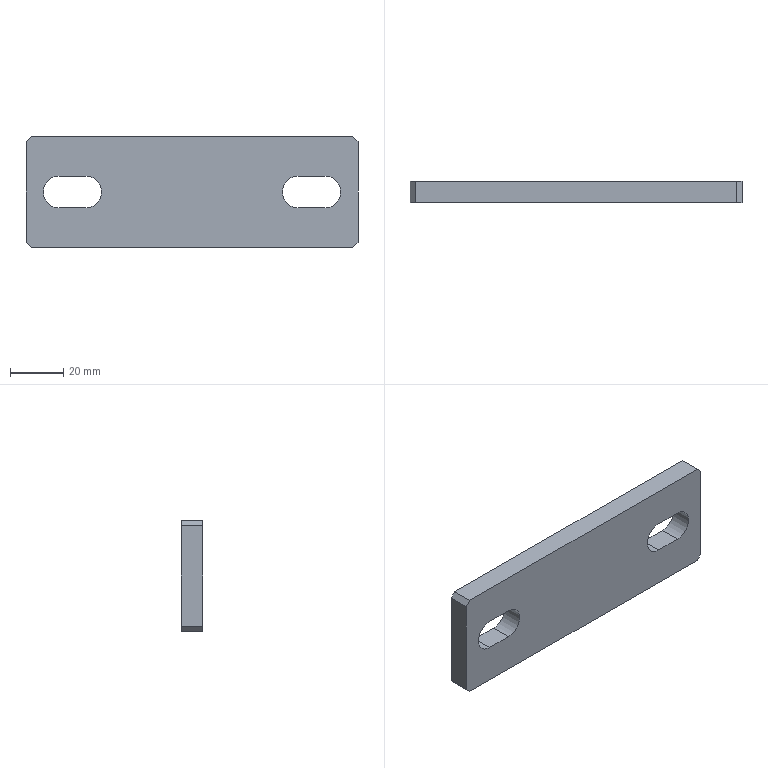Part | STEP file | 楼梯护栏连接Plate 1 | 1 solid | 18 faces | box 125 x 8 x 42 mm | volume 38206 mm3 | plane 14 | cylinder 4 | commonest cylinder face diameters 12 x4
STEP:
#1=CARTESIAN_POINT('',(0.,0.,0.));
#2=DIRECTION('',(0.,0.,1.));
#3=DIRECTION('',(1.,0.,0.));
#4=AXIS2_PLACEMENT_3D('',#1,#2,#3);
#5=CARTESIAN_POINT('',(-60.5,8.,21.));
#6=VERTEX_POINT('',#5);
#7=CARTESIAN_POINT('',(60.5,8.,21.));
#8=VERTEX_POINT('',#7);
#9=CARTESIAN_POINT('',(-62.5,8.,21.));
#10=DIRECTION('',(1.,0.,0.));
#11=VECTOR('',#10,1.);
#12=LINE('',#9,#11);
#13=CARTESIAN_POINT('',(0.,8.,0.));
#14=DIRECTION('',(0.,1.,0.));
#15=DIRECTION('',(0.,0.,1.));
#16=AXIS2_PLACEMENT_3D('',#13,#14,#15);
#17=PLANE('',#16);
#18=CARTESIAN_POINT('',(21.,-62.5));
#19=DIRECTION('',(0.,1.));
#20=VECTOR('',#19,1.);
#21=LINE('',#18,#20);
#22=(GEOMETRIC_REPRESENTATION_CONTEXT(2)PARAMETRIC_REPRESENTATION_CONTEXT()REPRESENTATION_CONTEXT('',''));
#23=DEFINITIONAL_REPRESENTATION('',(#21),#22);
#24=PCURVE('',#17,#23);
#25=CARTESIAN_POINT('',(-62.5,8.,21.));
#26=DIRECTION('',(0.,0.,-1.));
#27=DIRECTION('',(-1.,0.,0.));
#28=AXIS2_PLACEMENT_3D('',#25,#26,#27);
#29=PLANE('',#28);
#30=CARTESIAN_POINT('',(0.,0.));
#31=DIRECTION('',(-1.,0.));
#32=VECTOR('',#31,1.);
#33=LINE('',#30,#32);
#34=(GEOMETRIC_REPRESENTATION_CONTEXT(2)PARAMETRIC_REPRESENTATION_CONTEXT()REPRESENTATION_CONTEXT('',''));
#35=DEFINITIONAL_REPRESENTATION('',(#33),#34);
#36=PCURVE('',#29,#35);
#37=SURFACE_CURVE('',#12,(#24,#36),.PCURVE_S1.);
#38=EDGE_CURVE('',#6,#8,#37,.T.);
#39=ORIENTED_EDGE('',*,*,#38,.T.);
#40=CARTESIAN_POINT('',(62.5,8.,19.));
#41=VERTEX_POINT('',#40);
#42=CARTESIAN_POINT('',(40.75,8.,40.75));
#43=DIRECTION('',(0.7071,0.,-0.7071));
#44=VECTOR('',#43,1.);
#45=LINE('',#42,#44);
#46=CARTESIAN_POINT('',(40.75,40.75));
#47=DIRECTION('',(-0.7071,0.7071));
#48=VECTOR('',#47,1.);
#49=LINE('',#46,#48);
#50=(GEOMETRIC_REPRESENTATION_CONTEXT(2)PARAMETRIC_REPRESENTATION_CONTEXT()REPRESENTATION_CONTEXT('',''));
#51=DEFINITIONAL_REPRESENTATION('',(#49),#50);
#52=PCURVE('',#17,#51);
#53=CARTESIAN_POINT('',(62.5,8.,19.));
#54=DIRECTION('',(-0.7071,0.,-0.7071));
#55=DIRECTION('',(0.,-1.,0.));
#56=AXIS2_PLACEMENT_3D('',#53,#54,#55);
#57=PLANE('',#56);
#58=CARTESIAN_POINT('',(0.,30.759));
#59=DIRECTION('',(0.,-1.));
#60=VECTOR('',#59,1.);
#61=LINE('',#58,#60);
#62=(GEOMETRIC_REPRESENTATION_CONTEXT(2)PARAMETRIC_REPRESENTATION_CONTEXT()REPRESENTATION_CONTEXT('',''));
#63=DEFINITIONAL_REPRESENTATION('',(#61),#62);
#64=PCURVE('',#57,#63);
#65=SURFACE_CURVE('',#45,(#52,#64),.PCURVE_S1.);
#66=EDGE_CURVE('',#8,#41,#65,.T.);
#67=ORIENTED_EDGE('',*,*,#66,.T.);
#68=CARTESIAN_POINT('',(62.5,8.,-19.));
#69=VERTEX_POINT('',#68);
#70=CARTESIAN_POINT('',(62.5,8.,-21.));
#71=DIRECTION('',(0.,0.,-1.));
#72=VECTOR('',#71,1.);
#73=LINE('',#70,#72);
#74=CARTESIAN_POINT('',(-21.,62.5));
#75=DIRECTION('',(-1.,0.));
#76=VECTOR('',#75,1.);
#77=LINE('',#74,#76);
#78=(GEOMETRIC_REPRESENTATION_CONTEXT(2)PARAMETRIC_REPRESENTATION_CONTEXT()REPRESENTATION_CONTEXT('',''));
#79=DEFINITIONAL_REPRESENTATION('',(#77),#78);
#80=PCURVE('',#17,#79);
#81=CARTESIAN_POINT('',(62.5,8.,-21.));
#82=DIRECTION('',(-1.,0.,0.));
#83=DIRECTION('',(0.,0.,1.));
#84=AXIS2_PLACEMENT_3D('',#81,#82,#83);
#85=PLANE('',#84);
#86=CARTESIAN_POINT('',(0.,0.));
#87=DIRECTION('',(-1.,0.));
#88=VECTOR('',#87,1.);
#89=LINE('',#86,#88);
#90=(GEOMETRIC_REPRESENTATION_CONTEXT(2)PARAMETRIC_REPRESENTATION_CONTEXT()REPRESENTATION_CONTEXT('',''));
#91=DEFINITIONAL_REPRESENTATION('',(#89),#90);
#92=PCURVE('',#85,#91);
#93=SURFACE_CURVE('',#73,(#80,#92),.PCURVE_S1.);
#94=EDGE_CURVE('',#41,#69,#93,.T.);
#95=ORIENTED_EDGE('',*,*,#94,.T.);
#96=CARTESIAN_POINT('',(60.5,8.,-21.));
#97=VERTEX_POINT('',#96);
#98=CARTESIAN_POINT('',(40.75,8.,-40.75));
#99=DIRECTION('',(-0.7071,0.,-0.7071));
#100=VECTOR('',#99,1.);
#101=LINE('',#98,#100);
#102=CARTESIAN_POINT('',(-40.75,40.75));
#103=DIRECTION('',(-0.7071,-0.7071));
#104=VECTOR('',#103,1.);
#105=LINE('',#102,#104);
#106=(GEOMETRIC_REPRESENTATION_CONTEXT(2)PARAMETRIC_REPRESENTATION_CONTEXT()REPRESENTATION_CONTEXT('',''));
#107=DEFINITIONAL_REPRESENTATION('',(#105),#106);
#108=PCURVE('',#17,#107);
#109=CARTESIAN_POINT('',(60.5,8.,-21.));
#110=DIRECTION('',(-0.7071,0.,0.7071));
#111=DIRECTION('',(0.,-1.,0.));
#112=AXIS2_PLACEMENT_3D('',#109,#110,#111);
#113=PLANE('',#112);
#114=CARTESIAN_POINT('',(0.,-27.931));
#115=DIRECTION('',(0.,-1.));
#116=VECTOR('',#115,1.);
#117=LINE('',#114,#116);
#118=(GEOMETRIC_REPRESENTATION_CONTEXT(2)PARAMETRIC_REPRESENTATION_CONTEXT()REPRESENTATION_CONTEXT('',''));
#119=DEFINITIONAL_REPRESENTATION('',(#117),#118);
#120=PCURVE('',#113,#119);
#121=SURFACE_CURVE('',#101,(#108,#120),.PCURVE_S1.);
#122=EDGE_CURVE('',#69,#97,#121,.T.);
#123=ORIENTED_EDGE('',*,*,#122,.T.);
#124=CARTESIAN_POINT('',(-60.5,8.,-21.));
#125=VERTEX_POINT('',#124);
#126=CARTESIAN_POINT('',(-62.5,8.,-21.));
#127=DIRECTION('',(-1.,0.,0.));
#128=VECTOR('',#127,1.);
#129=LINE('',#126,#128);
#130=CARTESIAN_POINT('',(-21.,-62.5));
#131=DIRECTION('',(0.,-1.));
#132=VECTOR('',#131,1.);
#133=LINE('',#130,#132);
#134=(GEOMETRIC_REPRESENTATION_CONTEXT(2)PARAMETRIC_REPRESENTATION_CONTEXT()REPRESENTATION_CONTEXT('',''));
#135=DEFINITIONAL_REPRESENTATION('',(#133),#134);
#136=PCURVE('',#17,#135);
#137=CARTESIAN_POINT('',(-62.5,8.,-21.));
#138=DIRECTION('',(0.,0.,1.));
#139=DIRECTION('',(1.,0.,0.));
#140=AXIS2_PLACEMENT_3D('',#137,#138,#139);
#141=PLANE('',#140);
#142=CARTESIAN_POINT('',(0.,0.));
#143=DIRECTION('',(-1.,0.));
#144=VECTOR('',#143,1.);
#145=LINE('',#142,#144);
#146=(GEOMETRIC_REPRESENTATION_CONTEXT(2)PARAMETRIC_REPRESENTATION_CONTEXT()REPRESENTATION_CONTEXT('',''));
#147=DEFINITIONAL_REPRESENTATION('',(#145),#146);
#148=PCURVE('',#141,#147);
#149=SURFACE_CURVE('',#129,(#136,#148),.PCURVE_S1.);
#150=EDGE_CURVE('',#97,#125,#149,.T.);
#151=ORIENTED_EDGE('',*,*,#150,.T.);
#152=CARTESIAN_POINT('',(-62.5,8.,-19.));
#153=VERTEX_POINT('',#152);
#154=CARTESIAN_POINT('',(-40.75,8.,-40.75));
#155=DIRECTION('',(-0.7071,0.,0.7071));
#156=VECTOR('',#155,1.);
#157=LINE('',#154,#156);
#158=CARTESIAN_POINT('',(-40.75,-40.75));
#159=DIRECTION('',(0.7071,-0.7071));
#160=VECTOR('',#159,1.);
#161=LINE('',#158,#160);
#162=(GEOMETRIC_REPRESENTATION_CONTEXT(2)PARAMETRIC_REPRESENTATION_CONTEXT()REPRESENTATION_CONTEXT('',''));
#163=DEFINITIONAL_REPRESENTATION('',(#161),#162);
#164=PCURVE('',#17,#163);
#165=CARTESIAN_POINT('',(-62.5,8.,-19.));
#166=DIRECTION('',(0.7071,0.,0.7071));
#167=DIRECTION('',(0.,-1.,0.));
#168=AXIS2_PLACEMENT_3D('',#165,#166,#167);
#169=PLANE('',#168);
#170=CARTESIAN_POINT('',(0.,30.759));
#171=DIRECTION('',(0.,-1.));
#172=VECTOR('',#171,1.);
#173=LINE('',#170,#172);
#174=(GEOMETRIC_REPRESENTATION_CONTEXT(2)PARAMETRIC_REPRESENTATION_CONTEXT()REPRESENTATION_CONTEXT('',''));
#175=DEFINITIONAL_REPRESENTATION('',(#173),#174);
#176=PCURVE('',#169,#175);
#177=SURFACE_CURVE('',#157,(#164,#176),.PCURVE_S1.);
#178=EDGE_CURVE('',#125,#153,#177,.T.);
#179=ORIENTED_EDGE('',*,*,#178,.T.);
#180=CARTESIAN_POINT('',(-62.5,8.,19.));
#181=VERTEX_POINT('',#180);
#182=CARTESIAN_POINT('',(-62.5,8.,-21.));
#183=DIRECTION('',(0.,0.,1.));
#184=VECTOR('',#183,1.);
#185=LINE('',#182,#184);
#186=CARTESIAN_POINT('',(-21.,-62.5));
#187=DIRECTION('',(1.,0.));
#188=VECTOR('',#187,1.);
#189=LINE('',#186,#188);
#190=(GEOMETRIC_REPRESENTATION_CONTEXT(2)PARAMETRIC_REPRESENTATION_CONTEXT()REPRESENTATION_CONTEXT('',''));
#191=DEFINITIONAL_REPRESENTATION('',(#189),#190);
#192=PCURVE('',#17,#191);
#193=CARTESIAN_POINT('',(-62.5,8.,-21.));
#194=DIRECTION('',(1.,0.,0.));
#195=DIRECTION('',(0.,0.,-1.));
#196=AXIS2_PLACEMENT_3D('',#193,#194,#195);
#197=PLANE('',#196);
#198=CARTESIAN_POINT('',(0.,0.));
#199=DIRECTION('',(-1.,0.));
#200=VECTOR('',#199,1.);
#201=LINE('',#198,#200);
#202=(GEOMETRIC_REPRESENTATION_CONTEXT(2)PARAMETRIC_REPRESENTATION_CONTEXT()REPRESENTATION_CONTEXT('',''));
#203=DEFINITIONAL_REPRESENTATION('',(#201),#202);
#204=PCURVE('',#197,#203);
#205=SURFACE_CURVE('',#185,(#192,#204),.PCURVE_S1.);
#206=EDGE_CURVE('',#153,#181,#205,.T.);
#207=ORIENTED_EDGE('',*,*,#206,.T.);
#208=CARTESIAN_POINT('',(-40.75,8.,40.75));
#209=DIRECTION('',(0.7071,0.,0.7071));
#210=VECTOR('',#209,1.);
#211=LINE('',#208,#210);
#212=CARTESIAN_POINT('',(40.75,-40.75));
#213=DIRECTION('',(0.7071,0.7071));
#214=VECTOR('',#213,1.);
#215=LINE('',#212,#214);
#216=(GEOMETRIC_REPRESENTATION_CONTEXT(2)PARAMETRIC_REPRESENTATION_CONTEXT()REPRESENTATION_CONTEXT('',''));
#217=DEFINITIONAL_REPRESENTATION('',(#215),#216);
#218=PCURVE('',#17,#217);
#219=CARTESIAN_POINT('',(-60.5,8.,21.));
#220=DIRECTION('',(0.7071,0.,-0.7071));
#221=DIRECTION('',(0.,-1.,0.));
#222=AXIS2_PLACEMENT_3D('',#219,#220,#221);
#223=PLANE('',#222);
#224=CARTESIAN_POINT('',(0.,-27.931));
#225=DIRECTION('',(0.,-1.));
#226=VECTOR('',#225,1.);
#227=LINE('',#224,#226);
#228=(GEOMETRIC_REPRESENTATION_CONTEXT(2)PARAMETRIC_REPRESENTATION_CONTEXT()REPRESENTATION_CONTEXT('',''));
#229=DEFINITIONAL_REPRESENTATION('',(#227),#228);
#230=PCURVE('',#223,#229);
#231=SURFACE_CURVE('',#211,(#218,#230),.PCURVE_S1.);
#232=EDGE_CURVE('',#181,#6,#231,.T.);
#233=ORIENTED_EDGE('',*,*,#232,.T.);
#234=EDGE_LOOP('',(#39,#67,#95,#123,#151,#179,#207,#233));
#235=FACE_BOUND('',#234,.T.);
#236=CARTESIAN_POINT('',(40.,8.,-6.));
#237=VERTEX_POINT('',#236);
#238=CARTESIAN_POINT('',(40.,8.,6.));
#239=VERTEX_POINT('',#238);
#240=CARTESIAN_POINT('',(40.,8.,0.));
#241=DIRECTION('',(0.,1.,0.));
#242=DIRECTION('',(0.,0.,1.));
#243=AXIS2_PLACEMENT_3D('',#240,#241,#242);
#244=CIRCLE('',#243,6.);
#245=CARTESIAN_POINT('',(0.,40.));
#246=DIRECTION('',(1.,0.));
#247=AXIS2_PLACEMENT_2D('',#245,#246);
#248=CIRCLE('',#247,6.);
#249=(GEOMETRIC_REPRESENTATION_CONTEXT(2)PARAMETRIC_REPRESENTATION_CONTEXT()REPRESENTATION_CONTEXT('',''));
#250=DEFINITIONAL_REPRESENTATION('',(#248),#249);
#251=PCURVE('',#17,#250);
#252=CARTESIAN_POINT('',(40.,8.,0.));
#253=DIRECTION('',(0.,1.,0.));
#254=DIRECTION('',(0.,0.,1.));
#255=AXIS2_PLACEMENT_3D('',#252,#253,#254);
#256=CYLINDRICAL_SURFACE('',#255,6.);
#257=CARTESIAN_POINT('',(0.,0.));
#258=DIRECTION('',(1.,0.));
#259=VECTOR('',#258,1.);
#260=LINE('',#257,#259);
#261=(GEOMETRIC_REPRESENTATION_CONTEXT(2)PARAMETRIC_REPRESENTATION_CONTEXT()REPRESENTATION_CONTEXT('',''));
#262=DEFINITIONAL_REPRESENTATION('',(#260),#261);
#263=PCURVE('',#256,#262);
#264=SURFACE_CURVE('',#244,(#251,#263),.PCURVE_S1.);
#265=EDGE_CURVE('',#237,#239,#264,.T.);
#266=ORIENTED_EDGE('',*,*,#265,.F.);
#267=CARTESIAN_POINT('',(50.,8.,-6.));
#268=VERTEX_POINT('',#267);
#269=CARTESIAN_POINT('',(40.,8.,-6.));
#270=DIRECTION('',(1.,0.,0.));
#271=VECTOR('',#270,1.);
#272=LINE('',#269,#271);
#273=CARTESIAN_POINT('',(-6.,40.));
#274=DIRECTION('',(0.,1.));
#275=VECTOR('',#274,1.);
#276=LINE('',#273,#275);
#277=(GEOMETRIC_REPRESENTATION_CONTEXT(2)PARAMETRIC_REPRESENTATION_CONTEXT()REPRESENTATION_CONTEXT('',''));
#278=DEFINITIONAL_REPRESENTATION('',(#276),#277);
#279=PCURVE('',#17,#278);
#280=CARTESIAN_POINT('',(40.,8.,-6.));
#281=DIRECTION('',(0.,0.,-1.));
#282=DIRECTION('',(-1.,0.,0.));
#283=AXIS2_PLACEMENT_3D('',#280,#281,#282);
#284=PLANE('',#283);
#285=CARTESIAN_POINT('',(0.,0.));
#286=DIRECTION('',(-1.,0.));
#287=VECTOR('',#286,1.);
#288=LINE('',#285,#287);
#289=(GEOMETRIC_REPRESENTATION_CONTEXT(2)PARAMETRIC_REPRESENTATION_CONTEXT()REPRESENTATION_CONTEXT('',''));
#290=DEFINITIONAL_REPRESENTATION('',(#288),#289);
#291=PCURVE('',#284,#290);
#292=SURFACE_CURVE('',#272,(#279,#291),.PCURVE_S1.);
#293=EDGE_CURVE('',#237,#268,#292,.T.);
#294=ORIENTED_EDGE('',*,*,#293,.T.);
#295=CARTESIAN_POINT('',(50.,8.,6.));
#296=VERTEX_POINT('',#295);
#297=CARTESIAN_POINT('',(50.,8.,0.));
#298=DIRECTION('',(0.,1.,0.));
#299=DIRECTION('',(0.,0.,1.));
#300=AXIS2_PLACEMENT_3D('',#297,#298,#299);
#301=CIRCLE('',#300,6.);
#302=CARTESIAN_POINT('',(0.,50.));
#303=DIRECTION('',(1.,0.));
#304=AXIS2_PLACEMENT_2D('',#302,#303);
#305=CIRCLE('',#304,6.);
#306=(GEOMETRIC_REPRESENTATION_CONTEXT(2)PARAMETRIC_REPRESENTATION_CONTEXT()REPRESENTATION_CONTEXT('',''));
#307=DEFINITIONAL_REPRESENTATION('',(#305),#306);
#308=PCURVE('',#17,#307);
#309=CARTESIAN_POINT('',(50.,8.,0.));
#310=DIRECTION('',(0.,1.,0.));
#311=DIRECTION('',(0.,0.,1.));
#312=AXIS2_PLACEMENT_3D('',#309,#310,#311);
#313=CYLINDRICAL_SURFACE('',#312,6.);
#314=CARTESIAN_POINT('',(0.,0.));
#315=DIRECTION('',(1.,0.));
#316=VECTOR('',#315,1.);
#317=LINE('',#314,#316);
#318=(GEOMETRIC_REPRESENTATION_CONTEXT(2)PARAMETRIC_REPRESENTATION_CONTEXT()REPRESENTATION_CONTEXT('',''));
#319=DEFINITIONAL_REPRESENTATION('',(#317),#318);
#320=PCURVE('',#313,#319);
#321=SURFACE_CURVE('',#301,(#308,#320),.PCURVE_S1.);
#322=EDGE_CURVE('',#296,#268,#321,.T.);
#323=ORIENTED_EDGE('',*,*,#322,.F.);
#324=CARTESIAN_POINT('',(40.,8.,6.));
#325=DIRECTION('',(1.,0.,0.));
#326=VECTOR('',#325,1.);
#327=LINE('',#324,#326);
#328=CARTESIAN_POINT('',(6.,40.));
#329=DIRECTION('',(0.,1.));
#330=VECTOR('',#329,1.);
#331=LINE('',#328,#330);
#332=(GEOMETRIC_REPRESENTATION_CONTEXT(2)PARAMETRIC_REPRESENTATION_CONTEXT()REPRESENTATION_CONTEXT('',''));
#333=DEFINITIONAL_REPRESENTATION('',(#331),#332);
#334=PCURVE('',#17,#333);
#335=CARTESIAN_POINT('',(40.,8.,6.));
#336=DIRECTION('',(0.,0.,1.));
#337=DIRECTION('',(1.,0.,0.));
#338=AXIS2_PLACEMENT_3D('',#335,#336,#337);
#339=PLANE('',#338);
#340=CARTESIAN_POINT('',(0.,0.));
#341=DIRECTION('',(1.,0.));
#342=VECTOR('',#341,1.);
#343=LINE('',#340,#342);
#344=(GEOMETRIC_REPRESENTATION_CONTEXT(2)PARAMETRIC_REPRESENTATION_CONTEXT()REPRESENTATION_CONTEXT('',''));
#345=DEFINITIONAL_REPRESENTATION('',(#343),#344);
#346=PCURVE('',#339,#345);
#347=SURFACE_CURVE('',#327,(#334,#346),.PCURVE_S1.);
#348=EDGE_CURVE('',#239,#296,#347,.T.);
#349=ORIENTED_EDGE('',*,*,#348,.F.);
#350=EDGE_LOOP('',(#266,#294,#323,#349));
#351=FACE_BOUND('',#350,.T.);
#352=CARTESIAN_POINT('',(-50.,8.,-6.));
#353=VERTEX_POINT('',#352);
#354=CARTESIAN_POINT('',(-50.,8.,6.));
#355=VERTEX_POINT('',#354);
#356=CARTESIAN_POINT('',(-50.,8.,0.));
#357=DIRECTION('',(0.,1.,0.));
#358=DIRECTION('',(0.,0.,1.));
#359=AXIS2_PLACEMENT_3D('',#356,#357,#358);
#360=CIRCLE('',#359,6.);
#361=CARTESIAN_POINT('',(0.,-50.));
#362=DIRECTION('',(1.,0.));
#363=AXIS2_PLACEMENT_2D('',#361,#362);
#364=CIRCLE('',#363,6.);
#365=(GEOMETRIC_REPRESENTATION_CONTEXT(2)PARAMETRIC_REPRESENTATION_CONTEXT()REPRESENTATION_CONTEXT('',''));
#366=DEFINITIONAL_REPRESENTATION('',(#364),#365);
#367=PCURVE('',#17,#366);
#368=CARTESIAN_POINT('',(-50.,8.,0.));
#369=DIRECTION('',(0.,1.,0.));
#370=DIRECTION('',(0.,0.,1.));
#371=AXIS2_PLACEMENT_3D('',#368,#369,#370);
#372=CYLINDRICAL_SURFACE('',#371,6.);
#373=CARTESIAN_POINT('',(0.,0.));
#374=DIRECTION('',(1.,0.));
#375=VECTOR('',#374,1.);
#376=LINE('',#373,#375);
#377=(GEOMETRIC_REPRESENTATION_CONTEXT(2)PARAMETRIC_REPRESENTATION_CONTEXT()REPRESENTATION_CONTEXT('',''));
#378=DEFINITIONAL_REPRESENTATION('',(#376),#377);
#379=PCURVE('',#372,#378);
#380=SURFACE_CURVE('',#360,(#367,#379),.PCURVE_S1.);
#381=EDGE_CURVE('',#353,#355,#380,.T.);
#382=ORIENTED_EDGE('',*,*,#381,.F.);
#383=CARTESIAN_POINT('',(-40.,8.,-6.));
#384=VERTEX_POINT('',#383);
#385=CARTESIAN_POINT('',(-50.,8.,-6.));
#386=DIRECTION('',(1.,0.,0.));
#387=VECTOR('',#386,1.);
#388=LINE('',#385,#387);
#389=CARTESIAN_POINT('',(-6.,-50.));
#390=DIRECTION('',(0.,1.));
#391=VECTOR('',#390,1.);
#392=LINE('',#389,#391);
#393=(GEOMETRIC_REPRESENTATION_CONTEXT(2)PARAMETRIC_REPRESENTATION_CONTEXT()REPRESENTATION_CONTEXT('',''));
#394=DEFINITIONAL_REPRESENTATION('',(#392),#393);
#395=PCURVE('',#17,#394);
#396=CARTESIAN_POINT('',(-50.,8.,-6.));
#397=DIRECTION('',(0.,0.,-1.));
#398=DIRECTION('',(-1.,0.,0.));
#399=AXIS2_PLACEMENT_3D('',#396,#397,#398);
#400=PLANE('',#399);
#401=CARTESIAN_POINT('',(0.,0.));
#402=DIRECTION('',(-1.,0.));
#403=VECTOR('',#402,1.);
#404=LINE('',#401,#403);
#405=(GEOMETRIC_REPRESENTATION_CONTEXT(2)PARAMETRIC_REPRESENTATION_CONTEXT()REPRESENTATION_CONTEXT('',''));
#406=DEFINITIONAL_REPRESENTATION('',(#404),#405);
#407=PCURVE('',#400,#406);
#408=SURFACE_CURVE('',#388,(#395,#407),.PCURVE_S1.);
#409=EDGE_CURVE('',#353,#384,#408,.T.);
#410=ORIENTED_EDGE('',*,*,#409,.T.);
#411=CARTESIAN_POINT('',(-40.,8.,6.));
#412=VERTEX_POINT('',#411);
#413=CARTESIAN_POINT('',(-40.,8.,0.));
#414=DIRECTION('',(0.,1.,0.));
#415=DIRECTION('',(0.,0.,1.));
#416=AXIS2_PLACEMENT_3D('',#413,#414,#415);
#417=CIRCLE('',#416,6.);
#418=CARTESIAN_POINT('',(0.,-40.));
#419=DIRECTION('',(1.,0.));
#420=AXIS2_PLACEMENT_2D('',#418,#419);
#421=CIRCLE('',#420,6.);
#422=(GEOMETRIC_REPRESENTATION_CONTEXT(2)PARAMETRIC_REPRESENTATION_CONTEXT()REPRESENTATION_CONTEXT('',''));
#423=DEFINITIONAL_REPRESENTATION('',(#421),#422);
#424=PCURVE('',#17,#423);
#425=CARTESIAN_POINT('',(-40.,8.,0.));
#426=DIRECTION('',(0.,1.,0.));
#427=DIRECTION('',(0.,0.,1.));
#428=AXIS2_PLACEMENT_3D('',#425,#426,#427);
#429=CYLINDRICAL_SURFACE('',#428,6.);
#430=CARTESIAN_POINT('',(0.,0.));
#431=DIRECTION('',(1.,0.));
#432=VECTOR('',#431,1.);
#433=LINE('',#430,#432);
#434=(GEOMETRIC_REPRESENTATION_CONTEXT(2)PARAMETRIC_REPRESENTATION_CONTEXT()REPRESENTATION_CONTEXT('',''));
#435=DEFINITIONAL_REPRESENTATION('',(#433),#434);
#436=PCURVE('',#429,#435);
#437=SURFACE_CURVE('',#417,(#424,#436),.PCURVE_S1.);
#438=EDGE_CURVE('',#412,#384,#437,.T.);
#439=ORIENTED_EDGE('',*,*,#438,.F.);
#440=CARTESIAN_POINT('',(-50.,8.,6.));
#441=DIRECTION('',(1.,0.,0.));
#442=VECTOR('',#441,1.);
#443=LINE('',#440,#442);
#444=CARTESIAN_POINT('',(6.,-50.));
#445=DIRECTION('',(0.,1.));
#446=VECTOR('',#445,1.);
#447=LINE('',#444,#446);
#448=(GEOMETRIC_REPRESENTATION_CONTEXT(2)PARAMETRIC_REPRESENTATION_CONTEXT()REPRESENTATION_CONTEXT('',''));
#449=DEFINITIONAL_REPRESENTATION('',(#447),#448);
#450=PCURVE('',#17,#449);
#451=CARTESIAN_POINT('',(-50.,8.,6.));
#452=DIRECTION('',(0.,0.,1.));
#453=DIRECTION('',(1.,0.,0.));
#454=AXIS2_PLACEMENT_3D('',#451,#452,#453);
#455=PLANE('',#454);
#456=CARTESIAN_POINT('',(0.,0.));
#457=DIRECTION('',(1.,0.));
#458=VECTOR('',#457,1.);
#459=LINE('',#456,#458);
#460=(GEOMETRIC_REPRESENTATION_CONTEXT(2)PARAMETRIC_REPRESENTATION_CONTEXT()REPRESENTATION_CONTEXT('',''));
#461=DEFINITIONAL_REPRESENTATION('',(#459),#460);
#462=PCURVE('',#455,#461);
#463=SURFACE_CURVE('',#443,(#450,#462),.PCURVE_S1.);
#464=EDGE_CURVE('',#355,#412,#463,.T.);
#465=ORIENTED_EDGE('',*,*,#464,.F.);
#466=EDGE_LOOP('',(#382,#410,#439,#465));
#467=FACE_BOUND('',#466,.T.);
#468=ADVANCED_FACE('',(#235,#351,#467),#17,.T.);
#469=ORIENTED_EDGE('',*,*,#94,.F.);
#470=CARTESIAN_POINT('',(62.5,0.,19.));
#471=VERTEX_POINT('',#470);
#472=CARTESIAN_POINT('',(62.5,8.,19.));
#473=DIRECTION('',(0.,-1.,0.));
#474=VECTOR('',#473,1.);
#475=LINE('',#472,#474);
#476=CARTESIAN_POINT('',(40.,0.));
#477=DIRECTION('',(0.,-1.));
#478=VECTOR('',#477,1.);
#479=LINE('',#476,#478);
#480=(GEOMETRIC_REPRESENTATION_CONTEXT(2)PARAMETRIC_REPRESENTATION_CONTEXT()REPRESENTATION_CONTEXT('',''));
#481=DEFINITIONAL_REPRESENTATION('',(#479),#480);
#482=PCURVE('',#85,#481);
#483=CARTESIAN_POINT('',(0.,0.));
#484=DIRECTION('',(1.,0.));
#485=VECTOR('',#484,1.);
#486=LINE('',#483,#485);
#487=(GEOMETRIC_REPRESENTATION_CONTEXT(2)PARAMETRIC_REPRESENTATION_CONTEXT()REPRESENTATION_CONTEXT('',''));
#488=DEFINITIONAL_REPRESENTATION('',(#486),#487);
#489=PCURVE('',#57,#488);
#490=SURFACE_CURVE('',#475,(#482,#489),.PCURVE_S1.);
#491=EDGE_CURVE('',#41,#471,#490,.T.);
#492=ORIENTED_EDGE('',*,*,#491,.T.);
#493=CARTESIAN_POINT('',(62.5,0.,-19.));
#494=VERTEX_POINT('',#493);
#495=CARTESIAN_POINT('',(62.5,0.,-21.));
#496=DIRECTION('',(0.,0.,-1.));
#497=VECTOR('',#496,1.);
#498=LINE('',#495,#497);
#499=CARTESIAN_POINT('',(0.,-8.));
#500=DIRECTION('',(-1.,0.));
#501=VECTOR('',#500,1.);
#502=LINE('',#499,#501);
#503=(GEOMETRIC_REPRESENTATION_CONTEXT(2)PARAMETRIC_REPRESENTATION_CONTEXT()REPRESENTATION_CONTEXT('',''));
#504=DEFINITIONAL_REPRESENTATION('',(#502),#503);
#505=PCURVE('',#85,#504);
#506=CARTESIAN_POINT('',(0.,0.,0.));
#507=DIRECTION('',(0.,1.,0.));
#508=DIRECTION('',(0.,0.,1.));
#509=AXIS2_PLACEMENT_3D('',#506,#507,#508);
#510=PLANE('',#509);
#511=CARTESIAN_POINT('',(-21.,62.5));
#512=DIRECTION('',(-1.,0.));
#513=VECTOR('',#512,1.);
#514=LINE('',#511,#513);
#515=(GEOMETRIC_REPRESENTATION_CONTEXT(2)PARAMETRIC_REPRESENTATION_CONTEXT()REPRESENTATION_CONTEXT('',''));
#516=DEFINITIONAL_REPRESENTATION('',(#514),#515);
#517=PCURVE('',#510,#516);
#518=SURFACE_CURVE('',#498,(#505,#517),.PCURVE_S1.);
#519=EDGE_CURVE('',#471,#494,#518,.T.);
#520=ORIENTED_EDGE('',*,*,#519,.T.);
#521=CARTESIAN_POINT('',(62.5,8.,-19.));
#522=DIRECTION('',(0.,1.,0.));
#523=VECTOR('',#522,1.);
#524=LINE('',#521,#523);
#525=CARTESIAN_POINT('',(2.,0.));
#526=DIRECTION('',(0.,1.));
#527=VECTOR('',#526,1.);
#528=LINE('',#525,#527);
#529=(GEOMETRIC_REPRESENTATION_CONTEXT(2)PARAMETRIC_REPRESENTATION_CONTEXT()REPRESENTATION_CONTEXT('',''));
#530=DEFINITIONAL_REPRESENTATION('',(#528),#529);
#531=PCURVE('',#85,#530);
#532=CARTESIAN_POINT('',(0.,2.828));
#533=DIRECTION('',(-1.,0.));
#534=VECTOR('',#533,1.);
#535=LINE('',#532,#534);
#536=(GEOMETRIC_REPRESENTATION_CONTEXT(2)PARAMETRIC_REPRESENTATION_CONTEXT()REPRESENTATION_CONTEXT('',''));
#537=DEFINITIONAL_REPRESENTATION('',(#535),#536);
#538=PCURVE('',#113,#537);
#539=SURFACE_CURVE('',#524,(#531,#538),.PCURVE_S1.);
#540=EDGE_CURVE('',#494,#69,#539,.T.);
#541=ORIENTED_EDGE('',*,*,#540,.T.);
#542=EDGE_LOOP('',(#469,#492,#520,#541));
#543=FACE_BOUND('',#542,.T.);
#544=ADVANCED_FACE('',(#543),#85,.F.);
#545=ORIENTED_EDGE('',*,*,#150,.F.);
#546=CARTESIAN_POINT('',(60.5,0.,-21.));
#547=VERTEX_POINT('',#546);
#548=CARTESIAN_POINT('',(60.5,8.,-21.));
#549=DIRECTION('',(0.,-1.,0.));
#550=VECTOR('',#549,1.);
#551=LINE('',#548,#550);
#552=CARTESIAN_POINT('',(123.,0.));
#553=DIRECTION('',(0.,-1.));
#554=VECTOR('',#553,1.);
#555=LINE('',#552,#554);
#556=(GEOMETRIC_REPRESENTATION_CONTEXT(2)PARAMETRIC_REPRESENTATION_CONTEXT()REPRESENTATION_CONTEXT('',''));
#557=DEFINITIONAL_REPRESENTATION('',(#555),#556);
#558=PCURVE('',#141,#557);
#559=CARTESIAN_POINT('',(0.,0.));
#560=DIRECTION('',(1.,0.));
#561=VECTOR('',#560,1.);
#562=LINE('',#559,#561);
#563=(GEOMETRIC_REPRESENTATION_CONTEXT(2)PARAMETRIC_REPRESENTATION_CONTEXT()REPRESENTATION_CONTEXT('',''));
#564=DEFINITIONAL_REPRESENTATION('',(#562),#563);
#565=PCURVE('',#113,#564);
#566=SURFACE_CURVE('',#551,(#558,#565),.PCURVE_S1.);
#567=EDGE_CURVE('',#97,#547,#566,.T.);
#568=ORIENTED_EDGE('',*,*,#567,.T.);
#569=CARTESIAN_POINT('',(-60.5,0.,-21.));
#570=VERTEX_POINT('',#569);
#571=CARTESIAN_POINT('',(-62.5,0.,-21.));
#572=DIRECTION('',(-1.,0.,0.));
#573=VECTOR('',#572,1.);
#574=LINE('',#571,#573);
#575=CARTESIAN_POINT('',(0.,-8.));
#576=DIRECTION('',(-1.,0.));
#577=VECTOR('',#576,1.);
#578=LINE('',#575,#577);
#579=(GEOMETRIC_REPRESENTATION_CONTEXT(2)PARAMETRIC_REPRESENTATION_CONTEXT()REPRESENTATION_CONTEXT('',''));
#580=DEFINITIONAL_REPRESENTATION('',(#578),#579);
#581=PCURVE('',#141,#580);
#582=CARTESIAN_POINT('',(-21.,-62.5));
#583=DIRECTION('',(0.,-1.));
#584=VECTOR('',#583,1.);
#585=LINE('',#582,#584);
#586=(GEOMETRIC_REPRESENTATION_CONTEXT(2)PARAMETRIC_REPRESENTATION_CONTEXT()REPRESENTATION_CONTEXT('',''));
#587=DEFINITIONAL_REPRESENTATION('',(#585),#586);
#588=PCURVE('',#510,#587);
#589=SURFACE_CURVE('',#574,(#581,#588),.PCURVE_S1.);
#590=EDGE_CURVE('',#547,#570,#589,.T.);
#591=ORIENTED_EDGE('',*,*,#590,.T.);
#592=CARTESIAN_POINT('',(-60.5,8.,-21.));
#593=DIRECTION('',(0.,1.,0.));
#594=VECTOR('',#593,1.);
#595=LINE('',#592,#594);
#596=CARTESIAN_POINT('',(2.,0.));
#597=DIRECTION('',(0.,1.));
#598=VECTOR('',#597,1.);
#599=LINE('',#596,#598);
#600=(GEOMETRIC_REPRESENTATION_CONTEXT(2)PARAMETRIC_REPRESENTATION_CONTEXT()REPRESENTATION_CONTEXT('',''));
#601=DEFINITIONAL_REPRESENTATION('',(#599),#600);
#602=PCURVE('',#141,#601);
#603=CARTESIAN_POINT('',(0.,2.828));
#604=DIRECTION('',(-1.,0.));
#605=VECTOR('',#604,1.);
#606=LINE('',#603,#605);
#607=(GEOMETRIC_REPRESENTATION_CONTEXT(2)PARAMETRIC_REPRESENTATION_CONTEXT()REPRESENTATION_CONTEXT('',''));
#608=DEFINITIONAL_REPRESENTATION('',(#606),#607);
#609=PCURVE('',#169,#608);
#610=SURFACE_CURVE('',#595,(#602,#609),.PCURVE_S1.);
#611=EDGE_CURVE('',#570,#125,#610,.T.);
#612=ORIENTED_EDGE('',*,*,#611,.T.);
#613=EDGE_LOOP('',(#545,#568,#591,#612));
#614=FACE_BOUND('',#613,.T.);
#615=ADVANCED_FACE('',(#614),#141,.F.);
#616=ORIENTED_EDGE('',*,*,#206,.F.);
#617=CARTESIAN_POINT('',(-62.5,0.,-19.));
#618=VERTEX_POINT('',#617);
#619=CARTESIAN_POINT('',(-62.5,8.,-19.));
#620=DIRECTION('',(0.,-1.,0.));
#621=VECTOR('',#620,1.);
#622=LINE('',#619,#621);
#623=CARTESIAN_POINT('',(-2.,0.));
#624=DIRECTION('',(0.,-1.));
#625=VECTOR('',#624,1.);
#626=LINE('',#623,#625);
#627=(GEOMETRIC_REPRESENTATION_CONTEXT(2)PARAMETRIC_REPRESENTATION_CONTEXT()REPRESENTATION_CONTEXT('',''));
#628=DEFINITIONAL_REPRESENTATION('',(#626),#627);
#629=PCURVE('',#197,#628);
#630=CARTESIAN_POINT('',(0.,0.));
#631=DIRECTION('',(1.,0.));
#632=VECTOR('',#631,1.);
#633=LINE('',#630,#632);
#634=(GEOMETRIC_REPRESENTATION_CONTEXT(2)PARAMETRIC_REPRESENTATION_CONTEXT()REPRESENTATION_CONTEXT('',''));
#635=DEFINITIONAL_REPRESENTATION('',(#633),#634);
#636=PCURVE('',#169,#635);
#637=SURFACE_CURVE('',#622,(#629,#636),.PCURVE_S1.);
#638=EDGE_CURVE('',#153,#618,#637,.T.);
#639=ORIENTED_EDGE('',*,*,#638,.T.);
#640=CARTESIAN_POINT('',(-62.5,0.,19.));
#641=VERTEX_POINT('',#640);
#642=CARTESIAN_POINT('',(-62.5,0.,-21.));
#643=DIRECTION('',(0.,0.,1.));
#644=VECTOR('',#643,1.);
#645=LINE('',#642,#644);
#646=CARTESIAN_POINT('',(0.,-8.));
#647=DIRECTION('',(-1.,0.));
#648=VECTOR('',#647,1.);
#649=LINE('',#646,#648);
#650=(GEOMETRIC_REPRESENTATION_CONTEXT(2)PARAMETRIC_REPRESENTATION_CONTEXT()REPRESENTATION_CONTEXT('',''));
#651=DEFINITIONAL_REPRESENTATION('',(#649),#650);
#652=PCURVE('',#197,#651);
#653=CARTESIAN_POINT('',(-21.,-62.5));
#654=DIRECTION('',(1.,0.));
#655=VECTOR('',#654,1.);
#656=LINE('',#653,#655);
#657=(GEOMETRIC_REPRESENTATION_CONTEXT(2)PARAMETRIC_REPRESENTATION_CONTEXT()REPRESENTATION_CONTEXT('',''));
#658=DEFINITIONAL_REPRESENTATION('',(#656),#657);
#659=PCURVE('',#510,#658);
#660=SURFACE_CURVE('',#645,(#652,#659),.PCURVE_S1.);
#661=EDGE_CURVE('',#618,#641,#660,.T.);
#662=ORIENTED_EDGE('',*,*,#661,.T.);
#663=CARTESIAN_POINT('',(-62.5,8.,19.));
#664=DIRECTION('',(0.,1.,0.));
#665=VECTOR('',#664,1.);
#666=LINE('',#663,#665);
#667=CARTESIAN_POINT('',(-40.,0.));
#668=DIRECTION('',(0.,1.));
#669=VECTOR('',#668,1.);
#670=LINE('',#667,#669);
#671=(GEOMETRIC_REPRESENTATION_CONTEXT(2)PARAMETRIC_REPRESENTATION_CONTEXT()REPRESENTATION_CONTEXT('',''));
#672=DEFINITIONAL_REPRESENTATION('',(#670),#671);
#673=PCURVE('',#197,#672);
#674=CARTESIAN_POINT('',(0.,2.828));
#675=DIRECTION('',(-1.,0.));
#676=VECTOR('',#675,1.);
#677=LINE('',#674,#676);
#678=(GEOMETRIC_REPRESENTATION_CONTEXT(2)PARAMETRIC_REPRESENTATION_CONTEXT()REPRESENTATION_CONTEXT('',''));
#679=DEFINITIONAL_REPRESENTATION('',(#677),#678);
#680=PCURVE('',#223,#679);
#681=SURFACE_CURVE('',#666,(#673,#680),.PCURVE_S1.);
#682=EDGE_CURVE('',#641,#181,#681,.T.);
#683=ORIENTED_EDGE('',*,*,#682,.T.);
#684=EDGE_LOOP('',(#616,#639,#662,#683));
#685=FACE_BOUND('',#684,.T.);
#686=ADVANCED_FACE('',(#685),#197,.F.);
#687=CARTESIAN_POINT('',(-60.5,0.,21.));
#688=VERTEX_POINT('',#687);
#689=CARTESIAN_POINT('',(60.5,0.,21.));
#690=VERTEX_POINT('',#689);
#691=CARTESIAN_POINT('',(-62.5,0.,21.));
#692=DIRECTION('',(1.,0.,0.));
#693=VECTOR('',#692,1.);
#694=LINE('',#691,#693);
#695=CARTESIAN_POINT('',(0.,-8.));
#696=DIRECTION('',(-1.,0.));
#697=VECTOR('',#696,1.);
#698=LINE('',#695,#697);
#699=(GEOMETRIC_REPRESENTATION_CONTEXT(2)PARAMETRIC_REPRESENTATION_CONTEXT()REPRESENTATION_CONTEXT('',''));
#700=DEFINITIONAL_REPRESENTATION('',(#698),#699);
#701=PCURVE('',#29,#700);
#702=CARTESIAN_POINT('',(21.,-62.5));
#703=DIRECTION('',(0.,1.));
#704=VECTOR('',#703,1.);
#705=LINE('',#702,#704);
#706=(GEOMETRIC_REPRESENTATION_CONTEXT(2)PARAMETRIC_REPRESENTATION_CONTEXT()REPRESENTATION_CONTEXT('',''));
#707=DEFINITIONAL_REPRESENTATION('',(#705),#706);
#708=PCURVE('',#510,#707);
#709=SURFACE_CURVE('',#694,(#701,#708),.PCURVE_S1.);
#710=EDGE_CURVE('',#688,#690,#709,.T.);
#711=ORIENTED_EDGE('',*,*,#710,.T.);
#712=CARTESIAN_POINT('',(60.5,8.,21.));
#713=DIRECTION('',(0.,1.,0.));
#714=VECTOR('',#713,1.);
#715=LINE('',#712,#714);
#716=CARTESIAN_POINT('',(-123.,0.));
#717=DIRECTION('',(0.,1.));
#718=VECTOR('',#717,1.);
#719=LINE('',#716,#718);
#720=(GEOMETRIC_REPRESENTATION_CONTEXT(2)PARAMETRIC_REPRESENTATION_CONTEXT()REPRESENTATION_CONTEXT('',''));
#721=DEFINITIONAL_REPRESENTATION('',(#719),#720);
#722=PCURVE('',#29,#721);
#723=CARTESIAN_POINT('',(0.,2.828));
#724=DIRECTION('',(-1.,0.));
#725=VECTOR('',#724,1.);
#726=LINE('',#723,#725);
#727=(GEOMETRIC_REPRESENTATION_CONTEXT(2)PARAMETRIC_REPRESENTATION_CONTEXT()REPRESENTATION_CONTEXT('',''));
#728=DEFINITIONAL_REPRESENTATION('',(#726),#727);
#729=PCURVE('',#57,#728);
#730=SURFACE_CURVE('',#715,(#722,#729),.PCURVE_S1.);
#731=EDGE_CURVE('',#690,#8,#730,.T.);
#732=ORIENTED_EDGE('',*,*,#731,.T.);
#733=ORIENTED_EDGE('',*,*,#38,.F.);
#734=CARTESIAN_POINT('',(-60.5,8.,21.));
#735=DIRECTION('',(0.,-1.,0.));
#736=VECTOR('',#735,1.);
#737=LINE('',#734,#736);
#738=CARTESIAN_POINT('',(-2.,0.));
#739=DIRECTION('',(0.,-1.));
#740=VECTOR('',#739,1.);
#741=LINE('',#738,#740);
#742=(GEOMETRIC_REPRESENTATION_CONTEXT(2)PARAMETRIC_REPRESENTATION_CONTEXT()REPRESENTATION_CONTEXT('',''));
#743=DEFINITIONAL_REPRESENTATION('',(#741),#742);
#744=PCURVE('',#29,#743);
#745=CARTESIAN_POINT('',(0.,0.));
#746=DIRECTION('',(1.,0.));
#747=VECTOR('',#746,1.);
#748=LINE('',#745,#747);
#749=(GEOMETRIC_REPRESENTATION_CONTEXT(2)PARAMETRIC_REPRESENTATION_CONTEXT()REPRESENTATION_CONTEXT('',''));
#750=DEFINITIONAL_REPRESENTATION('',(#748),#749);
#751=PCURVE('',#223,#750);
#752=SURFACE_CURVE('',#737,(#744,#751),.PCURVE_S1.);
#753=EDGE_CURVE('',#6,#688,#752,.T.);
#754=ORIENTED_EDGE('',*,*,#753,.T.);
#755=EDGE_LOOP('',(#711,#732,#733,#754));
#756=FACE_BOUND('',#755,.T.);
#757=ADVANCED_FACE('',(#756),#29,.F.);
#758=CARTESIAN_POINT('',(-50.,0.,-6.));
#759=VERTEX_POINT('',#758);
#760=CARTESIAN_POINT('',(-50.,0.,6.));
#761=VERTEX_POINT('',#760);
#762=CARTESIAN_POINT('',(-50.,0.,0.));
#763=DIRECTION('',(0.,1.,0.));
#764=DIRECTION('',(0.,0.,1.));
#765=AXIS2_PLACEMENT_3D('',#762,#763,#764);
#766=CIRCLE('',#765,6.);
#767=CARTESIAN_POINT('',(0.,-50.));
#768=DIRECTION('',(1.,0.));
#769=AXIS2_PLACEMENT_2D('',#767,#768);
#770=CIRCLE('',#769,6.);
#771=(GEOMETRIC_REPRESENTATION_CONTEXT(2)PARAMETRIC_REPRESENTATION_CONTEXT()REPRESENTATION_CONTEXT('',''));
#772=DEFINITIONAL_REPRESENTATION('',(#770),#771);
#773=PCURVE('',#510,#772);
#774=CARTESIAN_POINT('',(0.,-8.));
#775=DIRECTION('',(1.,0.));
#776=VECTOR('',#775,1.);
#777=LINE('',#774,#776);
#778=(GEOMETRIC_REPRESENTATION_CONTEXT(2)PARAMETRIC_REPRESENTATION_CONTEXT()REPRESENTATION_CONTEXT('',''));
#779=DEFINITIONAL_REPRESENTATION('',(#777),#778);
#780=PCURVE('',#372,#779);
#781=SURFACE_CURVE('',#766,(#773,#780),.PCURVE_S1.);
#782=EDGE_CURVE('',#759,#761,#781,.T.);
#783=ORIENTED_EDGE('',*,*,#782,.T.);
#784=CARTESIAN_POINT('',(-40.,0.,6.));
#785=VERTEX_POINT('',#784);
#786=CARTESIAN_POINT('',(0.,0.,6.));
#787=DIRECTION('',(1.,0.,0.));
#788=VECTOR('',#787,1.);
#789=LINE('',#786,#788);
#790=CARTESIAN_POINT('',(6.,0.));
#791=DIRECTION('',(0.,1.));
#792=VECTOR('',#791,1.);
#793=LINE('',#790,#792);
#794=(GEOMETRIC_REPRESENTATION_CONTEXT(2)PARAMETRIC_REPRESENTATION_CONTEXT()REPRESENTATION_CONTEXT('',''));
#795=DEFINITIONAL_REPRESENTATION('',(#793),#794);
#796=PCURVE('',#510,#795);
#797=CARTESIAN_POINT('',(50.,-8.));
#798=DIRECTION('',(1.,0.));
#799=VECTOR('',#798,1.);
#800=LINE('',#797,#799);
#801=(GEOMETRIC_REPRESENTATION_CONTEXT(2)PARAMETRIC_REPRESENTATION_CONTEXT()REPRESENTATION_CONTEXT('',''));
#802=DEFINITIONAL_REPRESENTATION('',(#800),#801);
#803=PCURVE('',#455,#802);
#804=SURFACE_CURVE('',#789,(#796,#803),.PCURVE_S1.);
#805=EDGE_CURVE('',#761,#785,#804,.T.);
#806=ORIENTED_EDGE('',*,*,#805,.T.);
#807=CARTESIAN_POINT('',(-40.,0.,-6.));
#808=VERTEX_POINT('',#807);
#809=CARTESIAN_POINT('',(-40.,0.,0.));
#810=DIRECTION('',(0.,1.,0.));
#811=DIRECTION('',(0.,0.,1.));
#812=AXIS2_PLACEMENT_3D('',#809,#810,#811);
#813=CIRCLE('',#812,6.);
#814=CARTESIAN_POINT('',(0.,-40.));
#815=DIRECTION('',(1.,0.));
#816=AXIS2_PLACEMENT_2D('',#814,#815);
#817=CIRCLE('',#816,6.);
#818=(GEOMETRIC_REPRESENTATION_CONTEXT(2)PARAMETRIC_REPRESENTATION_CONTEXT()REPRESENTATION_CONTEXT('',''));
#819=DEFINITIONAL_REPRESENTATION('',(#817),#818);
#820=PCURVE('',#510,#819);
#821=CARTESIAN_POINT('',(0.,-8.));
#822=DIRECTION('',(1.,0.));
#823=VECTOR('',#822,1.);
#824=LINE('',#821,#823);
#825=(GEOMETRIC_REPRESENTATION_CONTEXT(2)PARAMETRIC_REPRESENTATION_CONTEXT()REPRESENTATION_CONTEXT('',''));
#826=DEFINITIONAL_REPRESENTATION('',(#824),#825);
#827=PCURVE('',#429,#826);
#828=SURFACE_CURVE('',#813,(#820,#827),.PCURVE_S1.);
#829=EDGE_CURVE('',#785,#808,#828,.T.);
#830=ORIENTED_EDGE('',*,*,#829,.T.);
#831=CARTESIAN_POINT('',(0.,0.,-6.));
#832=DIRECTION('',(-1.,0.,0.));
#833=VECTOR('',#832,1.);
#834=LINE('',#831,#833);
#835=CARTESIAN_POINT('',(-6.,0.));
#836=DIRECTION('',(0.,-1.));
#837=VECTOR('',#836,1.);
#838=LINE('',#835,#837);
#839=(GEOMETRIC_REPRESENTATION_CONTEXT(2)PARAMETRIC_REPRESENTATION_CONTEXT()REPRESENTATION_CONTEXT('',''));
#840=DEFINITIONAL_REPRESENTATION('',(#838),#839);
#841=PCURVE('',#510,#840);
#842=CARTESIAN_POINT('',(-50.,-8.));
#843=DIRECTION('',(1.,0.));
#844=VECTOR('',#843,1.);
#845=LINE('',#842,#844);
#846=(GEOMETRIC_REPRESENTATION_CONTEXT(2)PARAMETRIC_REPRESENTATION_CONTEXT()REPRESENTATION_CONTEXT('',''));
#847=DEFINITIONAL_REPRESENTATION('',(#845),#846);
#848=PCURVE('',#400,#847);
#849=SURFACE_CURVE('',#834,(#841,#848),.PCURVE_S1.);
#850=EDGE_CURVE('',#808,#759,#849,.T.);
#851=ORIENTED_EDGE('',*,*,#850,.T.);
#852=EDGE_LOOP('',(#783,#806,#830,#851));
#853=FACE_BOUND('',#852,.T.);
#854=CARTESIAN_POINT('',(40.,0.,6.));
#855=VERTEX_POINT('',#854);
#856=CARTESIAN_POINT('',(50.,0.,6.));
#857=VERTEX_POINT('',#856);
#858=CARTESIAN_POINT('',(0.,0.,6.));
#859=DIRECTION('',(1.,0.,0.));
#860=VECTOR('',#859,1.);
#861=LINE('',#858,#860);
#862=CARTESIAN_POINT('',(6.,0.));
#863=DIRECTION('',(0.,1.));
#864=VECTOR('',#863,1.);
#865=LINE('',#862,#864);
#866=(GEOMETRIC_REPRESENTATION_CONTEXT(2)PARAMETRIC_REPRESENTATION_CONTEXT()REPRESENTATION_CONTEXT('',''));
#867=DEFINITIONAL_REPRESENTATION('',(#865),#866);
#868=PCURVE('',#510,#867);
#869=CARTESIAN_POINT('',(-40.,-8.));
#870=DIRECTION('',(1.,0.));
#871=VECTOR('',#870,1.);
#872=LINE('',#869,#871);
#873=(GEOMETRIC_REPRESENTATION_CONTEXT(2)PARAMETRIC_REPRESENTATION_CONTEXT()REPRESENTATION_CONTEXT('',''));
#874=DEFINITIONAL_REPRESENTATION('',(#872),#873);
#875=PCURVE('',#339,#874);
#876=SURFACE_CURVE('',#861,(#868,#875),.PCURVE_S1.);
#877=EDGE_CURVE('',#855,#857,#876,.T.);
#878=ORIENTED_EDGE('',*,*,#877,.T.);
#879=CARTESIAN_POINT('',(50.,0.,-6.));
#880=VERTEX_POINT('',#879);
#881=CARTESIAN_POINT('',(50.,0.,0.));
#882=DIRECTION('',(0.,1.,0.));
#883=DIRECTION('',(0.,0.,1.));
#884=AXIS2_PLACEMENT_3D('',#881,#882,#883);
#885=CIRCLE('',#884,6.);
#886=CARTESIAN_POINT('',(0.,50.));
#887=DIRECTION('',(1.,0.));
#888=AXIS2_PLACEMENT_2D('',#886,#887);
#889=CIRCLE('',#888,6.);
#890=(GEOMETRIC_REPRESENTATION_CONTEXT(2)PARAMETRIC_REPRESENTATION_CONTEXT()REPRESENTATION_CONTEXT('',''));
#891=DEFINITIONAL_REPRESENTATION('',(#889),#890);
#892=PCURVE('',#510,#891);
#893=CARTESIAN_POINT('',(0.,-8.));
#894=DIRECTION('',(1.,0.));
#895=VECTOR('',#894,1.);
#896=LINE('',#893,#895);
#897=(GEOMETRIC_REPRESENTATION_CONTEXT(2)PARAMETRIC_REPRESENTATION_CONTEXT()REPRESENTATION_CONTEXT('',''));
#898=DEFINITIONAL_REPRESENTATION('',(#896),#897);
#899=PCURVE('',#313,#898);
#900=SURFACE_CURVE('',#885,(#892,#899),.PCURVE_S1.);
#901=EDGE_CURVE('',#857,#880,#900,.T.);
#902=ORIENTED_EDGE('',*,*,#901,.T.);
#903=CARTESIAN_POINT('',(40.,0.,-6.));
#904=VERTEX_POINT('',#903);
#905=CARTESIAN_POINT('',(0.,0.,-6.));
#906=DIRECTION('',(-1.,0.,0.));
#907=VECTOR('',#906,1.);
#908=LINE('',#905,#907);
#909=CARTESIAN_POINT('',(-6.,0.));
#910=DIRECTION('',(0.,-1.));
#911=VECTOR('',#910,1.);
#912=LINE('',#909,#911);
#913=(GEOMETRIC_REPRESENTATION_CONTEXT(2)PARAMETRIC_REPRESENTATION_CONTEXT()REPRESENTATION_CONTEXT('',''));
#914=DEFINITIONAL_REPRESENTATION('',(#912),#913);
#915=PCURVE('',#510,#914);
#916=CARTESIAN_POINT('',(40.,-8.));
#917=DIRECTION('',(1.,0.));
#918=VECTOR('',#917,1.);
#919=LINE('',#916,#918);
#920=(GEOMETRIC_REPRESENTATION_CONTEXT(2)PARAMETRIC_REPRESENTATION_CONTEXT()REPRESENTATION_CONTEXT('',''));
#921=DEFINITIONAL_REPRESENTATION('',(#919),#920);
#922=PCURVE('',#284,#921);
#923=SURFACE_CURVE('',#908,(#915,#922),.PCURVE_S1.);
#924=EDGE_CURVE('',#880,#904,#923,.T.);
#925=ORIENTED_EDGE('',*,*,#924,.T.);
#926=CARTESIAN_POINT('',(40.,0.,0.));
#927=DIRECTION('',(0.,1.,0.));
#928=DIRECTION('',(0.,0.,1.));
#929=AXIS2_PLACEMENT_3D('',#926,#927,#928);
#930=CIRCLE('',#929,6.);
#931=CARTESIAN_POINT('',(0.,40.));
#932=DIRECTION('',(1.,0.));
#933=AXIS2_PLACEMENT_2D('',#931,#932);
#934=CIRCLE('',#933,6.);
#935=(GEOMETRIC_REPRESENTATION_CONTEXT(2)PARAMETRIC_REPRESENTATION_CONTEXT()REPRESENTATION_CONTEXT('',''));
#936=DEFINITIONAL_REPRESENTATION('',(#934),#935);
#937=PCURVE('',#510,#936);
#938=CARTESIAN_POINT('',(0.,-8.));
#939=DIRECTION('',(1.,0.));
#940=VECTOR('',#939,1.);
#941=LINE('',#938,#940);
#942=(GEOMETRIC_REPRESENTATION_CONTEXT(2)PARAMETRIC_REPRESENTATION_CONTEXT()REPRESENTATION_CONTEXT('',''));
#943=DEFINITIONAL_REPRESENTATION('',(#941),#942);
#944=PCURVE('',#256,#943);
#945=SURFACE_CURVE('',#930,(#937,#944),.PCURVE_S1.);
#946=EDGE_CURVE('',#904,#855,#945,.T.);
#947=ORIENTED_EDGE('',*,*,#946,.T.);
#948=EDGE_LOOP('',(#878,#902,#925,#947));
#949=FACE_BOUND('',#948,.T.);
#950=ORIENTED_EDGE('',*,*,#519,.F.);
#951=CARTESIAN_POINT('',(62.5,0.,19.));
#952=DIRECTION('',(-0.7071,0.,0.7071));
#953=VECTOR('',#952,1.);
#954=LINE('',#951,#953);
#955=CARTESIAN_POINT('',(19.,62.5));
#956=DIRECTION('',(0.7071,-0.7071));
#957=VECTOR('',#956,1.);
#958=LINE('',#955,#957);
#959=(GEOMETRIC_REPRESENTATION_CONTEXT(2)PARAMETRIC_REPRESENTATION_CONTEXT()REPRESENTATION_CONTEXT('',''));
#960=DEFINITIONAL_REPRESENTATION('',(#958),#959);
#961=PCURVE('',#510,#960);
#962=CARTESIAN_POINT('',(8.,0.));
#963=DIRECTION('',(0.,1.));
#964=VECTOR('',#963,1.);
#965=LINE('',#962,#964);
#966=(GEOMETRIC_REPRESENTATION_CONTEXT(2)PARAMETRIC_REPRESENTATION_CONTEXT()REPRESENTATION_CONTEXT('',''));
#967=DEFINITIONAL_REPRESENTATION('',(#965),#966);
#968=PCURVE('',#57,#967);
#969=SURFACE_CURVE('',#954,(#961,#968),.PCURVE_S1.);
#970=EDGE_CURVE('',#471,#690,#969,.T.);
#971=ORIENTED_EDGE('',*,*,#970,.T.);
#972=ORIENTED_EDGE('',*,*,#710,.F.);
#973=CARTESIAN_POINT('',(-60.5,0.,21.));
#974=DIRECTION('',(-0.7071,0.,-0.7071));
#975=VECTOR('',#974,1.);
#976=LINE('',#973,#975);
#977=CARTESIAN_POINT('',(21.,-60.5));
#978=DIRECTION('',(-0.7071,-0.7071));
#979=VECTOR('',#978,1.);
#980=LINE('',#977,#979);
#981=(GEOMETRIC_REPRESENTATION_CONTEXT(2)PARAMETRIC_REPRESENTATION_CONTEXT()REPRESENTATION_CONTEXT('',''));
#982=DEFINITIONAL_REPRESENTATION('',(#980),#981);
#983=PCURVE('',#510,#982);
#984=CARTESIAN_POINT('',(8.,0.));
#985=DIRECTION('',(0.,1.));
#986=VECTOR('',#985,1.);
#987=LINE('',#984,#986);
#988=(GEOMETRIC_REPRESENTATION_CONTEXT(2)PARAMETRIC_REPRESENTATION_CONTEXT()REPRESENTATION_CONTEXT('',''));
#989=DEFINITIONAL_REPRESENTATION('',(#987),#988);
#990=PCURVE('',#223,#989);
#991=SURFACE_CURVE('',#976,(#983,#990),.PCURVE_S1.);
#992=EDGE_CURVE('',#688,#641,#991,.T.);
#993=ORIENTED_EDGE('',*,*,#992,.T.);
#994=ORIENTED_EDGE('',*,*,#661,.F.);
#995=CARTESIAN_POINT('',(-62.5,0.,-19.));
#996=DIRECTION('',(0.7071,0.,-0.7071));
#997=VECTOR('',#996,1.);
#998=LINE('',#995,#997);
#999=CARTESIAN_POINT('',(-19.,-62.5));
#1000=DIRECTION('',(-0.7071,0.7071));
#1001=VECTOR('',#1000,1.);
#1002=LINE('',#999,#1001);
#1003=(GEOMETRIC_REPRESENTATION_CONTEXT(2)PARAMETRIC_REPRESENTATION_CONTEXT()REPRESENTATION_CONTEXT('',''));
#1004=DEFINITIONAL_REPRESENTATION('',(#1002),#1003);
#1005=PCURVE('',#510,#1004);
#1006=CARTESIAN_POINT('',(8.,0.));
#1007=DIRECTION('',(0.,1.));
#1008=VECTOR('',#1007,1.);
#1009=LINE('',#1006,#1008);
#1010=(GEOMETRIC_REPRESENTATION_CONTEXT(2)PARAMETRIC_REPRESENTATION_CONTEXT()REPRESENTATION_CONTEXT('',''));
#1011=DEFINITIONAL_REPRESENTATION('',(#1009),#1010);
#1012=PCURVE('',#169,#1011);
#1013=SURFACE_CURVE('',#998,(#1005,#1012),.PCURVE_S1.);
#1014=EDGE_CURVE('',#618,#570,#1013,.T.);
#1015=ORIENTED_EDGE('',*,*,#1014,.T.);
#1016=ORIENTED_EDGE('',*,*,#590,.F.);
#1017=CARTESIAN_POINT('',(60.5,0.,-21.));
#1018=DIRECTION('',(0.7071,0.,0.7071));
#1019=VECTOR('',#1018,1.);
#1020=LINE('',#1017,#1019);
#1021=CARTESIAN_POINT('',(-21.,60.5));
#1022=DIRECTION('',(0.7071,0.7071));
#1023=VECTOR('',#1022,1.);
#1024=LINE('',#1021,#1023);
#1025=(GEOMETRIC_REPRESENTATION_CONTEXT(2)PARAMETRIC_REPRESENTATION_CONTEXT()REPRESENTATION_CONTEXT('',''));
#1026=DEFINITIONAL_REPRESENTATION('',(#1024),#1025);
#1027=PCURVE('',#510,#1026);
#1028=CARTESIAN_POINT('',(8.,0.));
#1029=DIRECTION('',(0.,1.));
#1030=VECTOR('',#1029,1.);
#1031=LINE('',#1028,#1030);
#1032=(GEOMETRIC_REPRESENTATION_CONTEXT(2)PARAMETRIC_REPRESENTATION_CONTEXT()REPRESENTATION_CONTEXT('',''));
#1033=DEFINITIONAL_REPRESENTATION('',(#1031),#1032);
#1034=PCURVE('',#113,#1033);
#1035=SURFACE_CURVE('',#1020,(#1027,#1034),.PCURVE_S1.);
#1036=EDGE_CURVE('',#547,#494,#1035,.T.);
#1037=ORIENTED_EDGE('',*,*,#1036,.T.);
#1038=EDGE_LOOP('',(#950,#971,#972,#993,#994,#1015,#1016,#1037));
#1039=FACE_BOUND('',#1038,.T.);
#1040=ADVANCED_FACE('',(#853,#949,#1039),#510,.F.);
#1041=ORIENTED_EDGE('',*,*,#901,.T.);
#1042=CARTESIAN_POINT('',(50.,8.,-6.));
#1043=DIRECTION('',(0.,1.,0.));
#1044=VECTOR('',#1043,1.);
#1045=LINE('',#1042,#1044);
#1046=CARTESIAN_POINT('',(3.142,0.));
#1047=DIRECTION('',(0.,1.));
#1048=VECTOR('',#1047,1.);
#1049=LINE('',#1046,#1048);
#1050=(GEOMETRIC_REPRESENTATION_CONTEXT(2)PARAMETRIC_REPRESENTATION_CONTEXT()REPRESENTATION_CONTEXT('',''));
#1051=DEFINITIONAL_REPRESENTATION('',(#1049),#1050);
#1052=PCURVE('',#313,#1051);
#1053=CARTESIAN_POINT('',(-10.,0.));
#1054=DIRECTION('',(0.,1.));
#1055=VECTOR('',#1054,1.);
#1056=LINE('',#1053,#1055);
#1057=(GEOMETRIC_REPRESENTATION_CONTEXT(2)PARAMETRIC_REPRESENTATION_CONTEXT()REPRESENTATION_CONTEXT('',''));
#1058=DEFINITIONAL_REPRESENTATION('',(#1056),#1057);
#1059=PCURVE('',#284,#1058);
#1060=SURFACE_CURVE('',#1045,(#1052,#1059),.PCURVE_S1.);
#1061=EDGE_CURVE('',#880,#268,#1060,.T.);
#1062=ORIENTED_EDGE('',*,*,#1061,.T.);
#1063=ORIENTED_EDGE('',*,*,#322,.F.);
#1064=CARTESIAN_POINT('',(50.,8.,6.));
#1065=DIRECTION('',(0.,-1.,0.));
#1066=VECTOR('',#1065,1.);
#1067=LINE('',#1064,#1066);
#1068=CARTESIAN_POINT('',(0.,0.));
#1069=DIRECTION('',(0.,-1.));
#1070=VECTOR('',#1069,1.);
#1071=LINE('',#1068,#1070);
#1072=(GEOMETRIC_REPRESENTATION_CONTEXT(2)PARAMETRIC_REPRESENTATION_CONTEXT()REPRESENTATION_CONTEXT('',''));
#1073=DEFINITIONAL_REPRESENTATION('',(#1071),#1072);
#1074=PCURVE('',#313,#1073);
#1075=CARTESIAN_POINT('',(10.,0.));
#1076=DIRECTION('',(0.,-1.));
#1077=VECTOR('',#1076,1.);
#1078=LINE('',#1075,#1077);
#1079=(GEOMETRIC_REPRESENTATION_CONTEXT(2)PARAMETRIC_REPRESENTATION_CONTEXT()REPRESENTATION_CONTEXT('',''));
#1080=DEFINITIONAL_REPRESENTATION('',(#1078),#1079);
#1081=PCURVE('',#339,#1080);
#1082=SURFACE_CURVE('',#1067,(#1074,#1081),.PCURVE_S1.);
#1083=EDGE_CURVE('',#296,#857,#1082,.T.);
#1084=ORIENTED_EDGE('',*,*,#1083,.T.);
#1085=EDGE_LOOP('',(#1041,#1062,#1063,#1084));
#1086=FACE_BOUND('',#1085,.F.);
#1087=ADVANCED_FACE('',(#1086),#313,.F.);
#1088=ORIENTED_EDGE('',*,*,#1061,.T.);
#1089=ORIENTED_EDGE('',*,*,#293,.F.);
#1090=CARTESIAN_POINT('',(40.,8.,-6.));
#1091=DIRECTION('',(0.,-1.,0.));
#1092=VECTOR('',#1091,1.);
#1093=LINE('',#1090,#1092);
#1094=CARTESIAN_POINT('',(0.,0.));
#1095=DIRECTION('',(0.,-1.));
#1096=VECTOR('',#1095,1.);
#1097=LINE('',#1094,#1096);
#1098=(GEOMETRIC_REPRESENTATION_CONTEXT(2)PARAMETRIC_REPRESENTATION_CONTEXT()REPRESENTATION_CONTEXT('',''));
#1099=DEFINITIONAL_REPRESENTATION('',(#1097),#1098);
#1100=PCURVE('',#284,#1099);
#1101=CARTESIAN_POINT('',(3.142,0.));
#1102=DIRECTION('',(0.,-1.));
#1103=VECTOR('',#1102,1.);
#1104=LINE('',#1101,#1103);
#1105=(GEOMETRIC_REPRESENTATION_CONTEXT(2)PARAMETRIC_REPRESENTATION_CONTEXT()REPRESENTATION_CONTEXT('',''));
#1106=DEFINITIONAL_REPRESENTATION('',(#1104),#1105);
#1107=PCURVE('',#256,#1106);
#1108=SURFACE_CURVE('',#1093,(#1100,#1107),.PCURVE_S1.);
#1109=EDGE_CURVE('',#237,#904,#1108,.T.);
#1110=ORIENTED_EDGE('',*,*,#1109,.T.);
#1111=ORIENTED_EDGE('',*,*,#924,.F.);
#1112=EDGE_LOOP('',(#1088,#1089,#1110,#1111));
#1113=FACE_BOUND('',#1112,.T.);
#1114=ADVANCED_FACE('',(#1113),#284,.F.);
#1115=ORIENTED_EDGE('',*,*,#946,.T.);
#1116=CARTESIAN_POINT('',(40.,8.,6.));
#1117=DIRECTION('',(0.,1.,0.));
#1118=VECTOR('',#1117,1.);
#1119=LINE('',#1116,#1118);
#1120=CARTESIAN_POINT('',(6.283,0.));
#1121=DIRECTION('',(0.,1.));
#1122=VECTOR('',#1121,1.);
#1123=LINE('',#1120,#1122);
#1124=(GEOMETRIC_REPRESENTATION_CONTEXT(2)PARAMETRIC_REPRESENTATION_CONTEXT()REPRESENTATION_CONTEXT('',''));
#1125=DEFINITIONAL_REPRESENTATION('',(#1123),#1124);
#1126=PCURVE('',#256,#1125);
#1127=CARTESIAN_POINT('',(0.,0.));
#1128=DIRECTION('',(0.,1.));
#1129=VECTOR('',#1128,1.);
#1130=LINE('',#1127,#1129);
#1131=(GEOMETRIC_REPRESENTATION_CONTEXT(2)PARAMETRIC_REPRESENTATION_CONTEXT()REPRESENTATION_CONTEXT('',''));
#1132=DEFINITIONAL_REPRESENTATION('',(#1130),#1131);
#1133=PCURVE('',#339,#1132);
#1134=SURFACE_CURVE('',#1119,(#1126,#1133),.PCURVE_S1.);
#1135=EDGE_CURVE('',#855,#239,#1134,.T.);
#1136=ORIENTED_EDGE('',*,*,#1135,.T.);
#1137=ORIENTED_EDGE('',*,*,#265,.F.);
#1138=ORIENTED_EDGE('',*,*,#1109,.T.);
#1139=EDGE_LOOP('',(#1115,#1136,#1137,#1138));
#1140=FACE_BOUND('',#1139,.F.);
#1141=ADVANCED_FACE('',(#1140),#256,.F.);
#1142=ORIENTED_EDGE('',*,*,#1135,.T.);
#1143=ORIENTED_EDGE('',*,*,#348,.T.);
#1144=ORIENTED_EDGE('',*,*,#1083,.T.);
#1145=ORIENTED_EDGE('',*,*,#877,.F.);
#1146=EDGE_LOOP('',(#1142,#1143,#1144,#1145));
#1147=FACE_BOUND('',#1146,.T.);
#1148=ADVANCED_FACE('',(#1147),#339,.F.);
#1149=CARTESIAN_POINT('',(-50.,8.,6.));
#1150=DIRECTION('',(0.,1.,0.));
#1151=VECTOR('',#1150,1.);
#1152=LINE('',#1149,#1151);
#1153=CARTESIAN_POINT('',(0.,0.));
#1154=DIRECTION('',(0.,1.));
#1155=VECTOR('',#1154,1.);
#1156=LINE('',#1153,#1155);
#1157=(GEOMETRIC_REPRESENTATION_CONTEXT(2)PARAMETRIC_REPRESENTATION_CONTEXT()REPRESENTATION_CONTEXT('',''));
#1158=DEFINITIONAL_REPRESENTATION('',(#1156),#1157);
#1159=PCURVE('',#455,#1158);
#1160=CARTESIAN_POINT('',(6.283,0.));
#1161=DIRECTION('',(0.,1.));
#1162=VECTOR('',#1161,1.);
#1163=LINE('',#1160,#1162);
#1164=(GEOMETRIC_REPRESENTATION_CONTEXT(2)PARAMETRIC_REPRESENTATION_CONTEXT()REPRESENTATION_CONTEXT('',''));
#1165=DEFINITIONAL_REPRESENTATION('',(#1163),#1164);
#1166=PCURVE('',#372,#1165);
#1167=SURFACE_CURVE('',#1152,(#1159,#1166),.PCURVE_S1.);
#1168=EDGE_CURVE('',#761,#355,#1167,.T.);
#1169=ORIENTED_EDGE('',*,*,#1168,.T.);
#1170=ORIENTED_EDGE('',*,*,#464,.T.);
#1171=CARTESIAN_POINT('',(-40.,8.,6.));
#1172=DIRECTION('',(0.,-1.,0.));
#1173=VECTOR('',#1172,1.);
#1174=LINE('',#1171,#1173);
#1175=CARTESIAN_POINT('',(10.,0.));
#1176=DIRECTION('',(0.,-1.));
#1177=VECTOR('',#1176,1.);
#1178=LINE('',#1175,#1177);
#1179=(GEOMETRIC_REPRESENTATION_CONTEXT(2)PARAMETRIC_REPRESENTATION_CONTEXT()REPRESENTATION_CONTEXT('',''));
#1180=DEFINITIONAL_REPRESENTATION('',(#1178),#1179);
#1181=PCURVE('',#455,#1180);
#1182=CARTESIAN_POINT('',(0.,0.));
#1183=DIRECTION('',(0.,-1.));
#1184=VECTOR('',#1183,1.);
#1185=LINE('',#1182,#1184);
#1186=(GEOMETRIC_REPRESENTATION_CONTEXT(2)PARAMETRIC_REPRESENTATION_CONTEXT()REPRESENTATION_CONTEXT('',''));
#1187=DEFINITIONAL_REPRESENTATION('',(#1185),#1186);
#1188=PCURVE('',#429,#1187);
#1189=SURFACE_CURVE('',#1174,(#1181,#1188),.PCURVE_S1.);
#1190=EDGE_CURVE('',#412,#785,#1189,.T.);
#1191=ORIENTED_EDGE('',*,*,#1190,.T.);
#1192=ORIENTED_EDGE('',*,*,#805,.F.);
#1193=EDGE_LOOP('',(#1169,#1170,#1191,#1192));
#1194=FACE_BOUND('',#1193,.T.);
#1195=ADVANCED_FACE('',(#1194),#455,.F.);
#1196=ORIENTED_EDGE('',*,*,#829,.T.);
#1197=CARTESIAN_POINT('',(-40.,8.,-6.));
#1198=DIRECTION('',(0.,1.,0.));
#1199=VECTOR('',#1198,1.);
#1200=LINE('',#1197,#1199);
#1201=CARTESIAN_POINT('',(3.142,0.));
#1202=DIRECTION('',(0.,1.));
#1203=VECTOR('',#1202,1.);
#1204=LINE('',#1201,#1203);
#1205=(GEOMETRIC_REPRESENTATION_CONTEXT(2)PARAMETRIC_REPRESENTATION_CONTEXT()REPRESENTATION_CONTEXT('',''));
#1206=DEFINITIONAL_REPRESENTATION('',(#1204),#1205);
#1207=PCURVE('',#429,#1206);
#1208=CARTESIAN_POINT('',(-10.,0.));
#1209=DIRECTION('',(0.,1.));
#1210=VECTOR('',#1209,1.);
#1211=LINE('',#1208,#1210);
#1212=(GEOMETRIC_REPRESENTATION_CONTEXT(2)PARAMETRIC_REPRESENTATION_CONTEXT()REPRESENTATION_CONTEXT('',''));
#1213=DEFINITIONAL_REPRESENTATION('',(#1211),#1212);
#1214=PCURVE('',#400,#1213);
#1215=SURFACE_CURVE('',#1200,(#1207,#1214),.PCURVE_S1.);
#1216=EDGE_CURVE('',#808,#384,#1215,.T.);
#1217=ORIENTED_EDGE('',*,*,#1216,.T.);
#1218=ORIENTED_EDGE('',*,*,#438,.F.);
#1219=ORIENTED_EDGE('',*,*,#1190,.T.);
#1220=EDGE_LOOP('',(#1196,#1217,#1218,#1219));
#1221=FACE_BOUND('',#1220,.F.);
#1222=ADVANCED_FACE('',(#1221),#429,.F.);
#1223=ORIENTED_EDGE('',*,*,#782,.T.);
#1224=ORIENTED_EDGE('',*,*,#1168,.T.);
#1225=ORIENTED_EDGE('',*,*,#381,.F.);
#1226=CARTESIAN_POINT('',(-50.,8.,-6.));
#1227=DIRECTION('',(0.,-1.,0.));
#1228=VECTOR('',#1227,1.);
#1229=LINE('',#1226,#1228);
#1230=CARTESIAN_POINT('',(3.142,0.));
#1231=DIRECTION('',(0.,-1.));
#1232=VECTOR('',#1231,1.);
#1233=LINE('',#1230,#1232);
#1234=(GEOMETRIC_REPRESENTATION_CONTEXT(2)PARAMETRIC_REPRESENTATION_CONTEXT()REPRESENTATION_CONTEXT('',''));
#1235=DEFINITIONAL_REPRESENTATION('',(#1233),#1234);
#1236=PCURVE('',#372,#1235);
#1237=CARTESIAN_POINT('',(0.,0.));
#1238=DIRECTION('',(0.,-1.));
#1239=VECTOR('',#1238,1.);
#1240=LINE('',#1237,#1239);
#1241=(GEOMETRIC_REPRESENTATION_CONTEXT(2)PARAMETRIC_REPRESENTATION_CONTEXT()REPRESENTATION_CONTEXT('',''));
#1242=DEFINITIONAL_REPRESENTATION('',(#1240),#1241);
#1243=PCURVE('',#400,#1242);
#1244=SURFACE_CURVE('',#1229,(#1236,#1243),.PCURVE_S1.);
#1245=EDGE_CURVE('',#353,#759,#1244,.T.);
#1246=ORIENTED_EDGE('',*,*,#1245,.T.);
#1247=EDGE_LOOP('',(#1223,#1224,#1225,#1246));
#1248=FACE_BOUND('',#1247,.F.);
#1249=ADVANCED_FACE('',(#1248),#372,.F.);
#1250=ORIENTED_EDGE('',*,*,#1216,.T.);
#1251=ORIENTED_EDGE('',*,*,#409,.F.);
#1252=ORIENTED_EDGE('',*,*,#1245,.T.);
#1253=ORIENTED_EDGE('',*,*,#850,.F.);
#1254=EDGE_LOOP('',(#1250,#1251,#1252,#1253));
#1255=FACE_BOUND('',#1254,.T.);
#1256=ADVANCED_FACE('',(#1255),#400,.F.);
#1257=ORIENTED_EDGE('',*,*,#66,.F.);
#1258=ORIENTED_EDGE('',*,*,#731,.F.);
#1259=ORIENTED_EDGE('',*,*,#970,.F.);
#1260=ORIENTED_EDGE('',*,*,#491,.F.);
#1261=EDGE_LOOP('',(#1257,#1258,#1259,#1260));
#1262=FACE_BOUND('',#1261,.T.);
#1263=ADVANCED_FACE('',(#1262),#57,.F.);
#1264=ORIENTED_EDGE('',*,*,#122,.F.);
#1265=ORIENTED_EDGE('',*,*,#540,.F.);
#1266=ORIENTED_EDGE('',*,*,#1036,.F.);
#1267=ORIENTED_EDGE('',*,*,#567,.F.);
#1268=EDGE_LOOP('',(#1264,#1265,#1266,#1267));
#1269=FACE_BOUND('',#1268,.T.);
#1270=ADVANCED_FACE('',(#1269),#113,.F.);
#1271=ORIENTED_EDGE('',*,*,#178,.F.);
#1272=ORIENTED_EDGE('',*,*,#611,.F.);
#1273=ORIENTED_EDGE('',*,*,#1014,.F.);
#1274=ORIENTED_EDGE('',*,*,#638,.F.);
#1275=EDGE_LOOP('',(#1271,#1272,#1273,#1274));
#1276=FACE_BOUND('',#1275,.T.);
#1277=ADVANCED_FACE('',(#1276),#169,.F.);
#1278=ORIENTED_EDGE('',*,*,#232,.F.);
#1279=ORIENTED_EDGE('',*,*,#682,.F.);
#1280=ORIENTED_EDGE('',*,*,#992,.F.);
#1281=ORIENTED_EDGE('',*,*,#753,.F.);
#1282=EDGE_LOOP('',(#1278,#1279,#1280,#1281));
#1283=FACE_BOUND('',#1282,.T.);
#1284=ADVANCED_FACE('',(#1283),#223,.F.);
#1285=CLOSED_SHELL('',(#468,#544,#615,#686,#757,#1040,#1087,#1114,#1141,#1148,#1195,#1222,#1249,#1256,#1263,#1270,#1277,#1284));
#1286=MANIFOLD_SOLID_BREP('',#1285);
#1287=(LENGTH_UNIT()NAMED_UNIT(*)SI_UNIT(.MILLI.,.METRE.));
#1288=UNCERTAINTY_MEASURE_WITH_UNIT(LENGTH_MEASURE(0.0000001),#1287,'','');
#1289=(NAMED_UNIT(*)PLANE_ANGLE_UNIT()SI_UNIT($,.RADIAN.));
#1290=(NAMED_UNIT(*)SI_UNIT($,.STERADIAN.)SOLID_ANGLE_UNIT());
#1291=(GEOMETRIC_REPRESENTATION_CONTEXT(3)GLOBAL_UNCERTAINTY_ASSIGNED_CONTEXT((#1288))GLOBAL_UNIT_ASSIGNED_CONTEXT((#1287,#1289,#1290))REPRESENTATION_CONTEXT('',''));
#1292=ADVANCED_BREP_SHAPE_REPRESENTATION('',(#4,#1286),#1291);